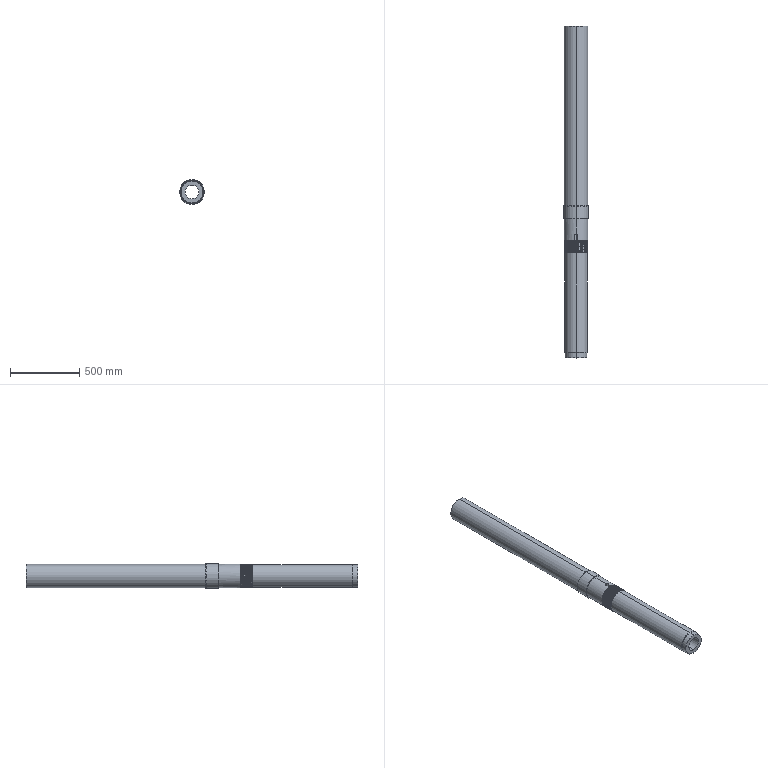Part | SolidWorks | features BaseBody 1 | 1 solid | 136 faces | box 180 x 2400 x 180 mm | volume 34786872 mm3 | cylinder 105 | cone 12 | plane 10 | spline 9 | commonest cylinder face diameters 170 x91 25 x2 100 x2 159.997 x2 165 x2 169.995 x2